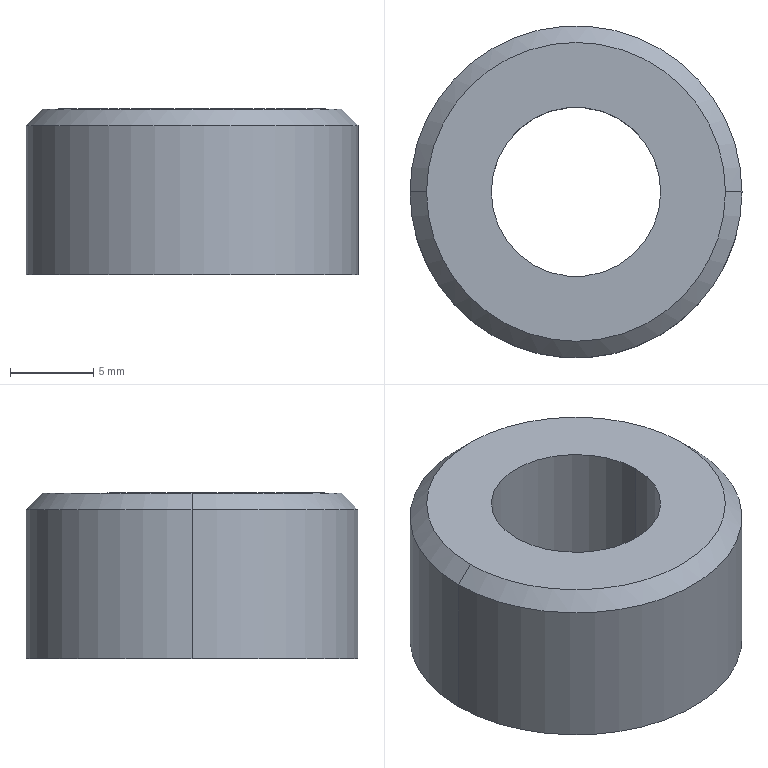Part | SolidWorks | features Chamfer 1, Extrusion 1, HoleWzd 1 | 1 solid | 8 faces | box 20 x 20 x 10 mm | volume 2294 mm3 | cylinder 4 | cone 2 | plane 2 | commonest cylinder face diameters 10.2 x2 20 x2
STEP:
#1=CARTESIAN_POINT('',(9.,0.,10.));
#2=VERTEX_POINT('',#1);
#3=CARTESIAN_POINT('',(-9.,0.,10.));
#4=VERTEX_POINT('',#3);
#5=CARTESIAN_POINT('',(0.,0.,10.));
#6=DIRECTION('',(0.,0.,1.));
#7=DIRECTION('',(1.,0.,0.));
#8=AXIS2_PLACEMENT_3D('',#5,#6,#7);
#9=CIRCLE('',#8,9.);
#10=EDGE_CURVE('',#2,#4,#9,.T.);
#11=ORIENTED_EDGE('',*,*,#10,.F.);
#12=CARTESIAN_POINT('',(10.,0.,9.));
#13=VERTEX_POINT('',#12);
#14=CARTESIAN_POINT('',(9.,0.,10.));
#15=DIRECTION('',(0.7071,0.,-0.7071));
#16=VECTOR('',#15,1000.);
#17=LINE('',#14,#16);
#18=EDGE_CURVE('',#2,#13,#17,.T.);
#19=ORIENTED_EDGE('',*,*,#18,.T.);
#20=CARTESIAN_POINT('',(-10.,0.,9.));
#21=VERTEX_POINT('',#20);
#22=CARTESIAN_POINT('',(0.,0.,9.));
#23=DIRECTION('',(0.,0.,-1.));
#24=DIRECTION('',(1.,0.,0.));
#25=AXIS2_PLACEMENT_3D('',#22,#23,#24);
#26=CIRCLE('',#25,10.);
#27=EDGE_CURVE('',#21,#13,#26,.T.);
#28=ORIENTED_EDGE('',*,*,#27,.F.);
#29=CARTESIAN_POINT('',(-9.,0.,10.));
#30=DIRECTION('',(-0.7071,0.,-0.7071));
#31=VECTOR('',#30,1000.);
#32=LINE('',#29,#31);
#33=EDGE_CURVE('',#4,#21,#32,.T.);
#34=ORIENTED_EDGE('',*,*,#33,.F.);
#35=EDGE_LOOP('',(#11,#19,#28,#34));
#36=FACE_OUTER_BOUND('',#35,.T.);
#37=CARTESIAN_POINT('',(0.,0.,10.));
#38=DIRECTION('',(0.,0.,-1.));
#39=DIRECTION('',(-1.,0.,0.));
#40=AXIS2_PLACEMENT_3D('',#37,#38,#39);
#41=CONICAL_SURFACE('',#40,9.,0.7854);
#42=ADVANCED_FACE('',(#36),#41,.T.);
#43=CARTESIAN_POINT('',(-5.1,0.,0.));
#44=VERTEX_POINT('',#43);
#45=CARTESIAN_POINT('',(5.1,0.,0.));
#46=VERTEX_POINT('',#45);
#47=CARTESIAN_POINT('',(0.,0.,0.));
#48=DIRECTION('',(0.,0.,1.));
#49=DIRECTION('',(1.,0.,0.));
#50=AXIS2_PLACEMENT_3D('',#47,#48,#49);
#51=CIRCLE('',#50,5.1);
#52=EDGE_CURVE('',#44,#46,#51,.T.);
#53=ORIENTED_EDGE('',*,*,#52,.F.);
#54=CARTESIAN_POINT('',(-5.1,0.,10.));
#55=VERTEX_POINT('',#54);
#56=CARTESIAN_POINT('',(-5.1,0.,10.));
#57=DIRECTION('',(0.,0.,1.));
#58=VECTOR('',#57,1000.);
#59=LINE('',#56,#58);
#60=EDGE_CURVE('',#44,#55,#59,.T.);
#61=ORIENTED_EDGE('',*,*,#60,.T.);
#62=CARTESIAN_POINT('',(5.1,0.,10.));
#63=VERTEX_POINT('',#62);
#64=CARTESIAN_POINT('',(0.,0.,10.));
#65=DIRECTION('',(0.,0.,1.));
#66=DIRECTION('',(1.,0.,0.));
#67=AXIS2_PLACEMENT_3D('',#64,#65,#66);
#68=CIRCLE('',#67,5.1);
#69=EDGE_CURVE('',#55,#63,#68,.T.);
#70=ORIENTED_EDGE('',*,*,#69,.T.);
#71=CARTESIAN_POINT('',(5.1,0.,10.));
#72=DIRECTION('',(0.,0.,1.));
#73=VECTOR('',#72,1000.);
#74=LINE('',#71,#73);
#75=EDGE_CURVE('',#46,#63,#74,.T.);
#76=ORIENTED_EDGE('',*,*,#75,.F.);
#77=EDGE_LOOP('',(#53,#61,#70,#76));
#78=FACE_OUTER_BOUND('',#77,.T.);
#79=CARTESIAN_POINT('',(0.,0.,10.));
#80=DIRECTION('',(0.,0.,1.));
#81=DIRECTION('',(1.,0.,0.));
#82=AXIS2_PLACEMENT_3D('',#79,#80,#81);
#83=CYLINDRICAL_SURFACE('',#82,5.1);
#84=ADVANCED_FACE('',(#78),#83,.F.);
#85=ORIENTED_EDGE('',*,*,#27,.T.);
#86=CARTESIAN_POINT('',(10.,0.,0.));
#87=VERTEX_POINT('',#86);
#88=CARTESIAN_POINT('',(10.,0.,10.));
#89=DIRECTION('',(0.,0.,-1.));
#90=VECTOR('',#89,1000.);
#91=LINE('',#88,#90);
#92=EDGE_CURVE('',#13,#87,#91,.T.);
#93=ORIENTED_EDGE('',*,*,#92,.T.);
#94=CARTESIAN_POINT('',(-10.,0.,0.));
#95=VERTEX_POINT('',#94);
#96=CARTESIAN_POINT('',(0.,0.,0.));
#97=DIRECTION('',(0.,0.,1.));
#98=DIRECTION('',(1.,0.,0.));
#99=AXIS2_PLACEMENT_3D('',#96,#97,#98);
#100=CIRCLE('',#99,10.);
#101=EDGE_CURVE('',#87,#95,#100,.T.);
#102=ORIENTED_EDGE('',*,*,#101,.T.);
#103=CARTESIAN_POINT('',(-10.,0.,10.));
#104=DIRECTION('',(0.,0.,-1.));
#105=VECTOR('',#104,1000.);
#106=LINE('',#103,#105);
#107=EDGE_CURVE('',#21,#95,#106,.T.);
#108=ORIENTED_EDGE('',*,*,#107,.F.);
#109=EDGE_LOOP('',(#85,#93,#102,#108));
#110=FACE_OUTER_BOUND('',#109,.T.);
#111=CARTESIAN_POINT('',(0.,0.,10.));
#112=DIRECTION('',(0.,0.,-1.));
#113=DIRECTION('',(-1.,0.,0.));
#114=AXIS2_PLACEMENT_3D('',#111,#112,#113);
#115=CYLINDRICAL_SURFACE('',#114,10.);
#116=ADVANCED_FACE('',(#110),#115,.T.);
#117=ORIENTED_EDGE('',*,*,#92,.F.);
#118=CARTESIAN_POINT('',(0.,0.,9.));
#119=DIRECTION('',(0.,0.,-1.));
#120=DIRECTION('',(1.,0.,0.));
#121=AXIS2_PLACEMENT_3D('',#118,#119,#120);
#122=CIRCLE('',#121,10.);
#123=EDGE_CURVE('',#13,#21,#122,.T.);
#124=ORIENTED_EDGE('',*,*,#123,.T.);
#125=ORIENTED_EDGE('',*,*,#107,.T.);
#126=CARTESIAN_POINT('',(0.,0.,0.));
#127=DIRECTION('',(0.,0.,1.));
#128=DIRECTION('',(1.,0.,0.));
#129=AXIS2_PLACEMENT_3D('',#126,#127,#128);
#130=CIRCLE('',#129,10.);
#131=EDGE_CURVE('',#95,#87,#130,.T.);
#132=ORIENTED_EDGE('',*,*,#131,.T.);
#133=EDGE_LOOP('',(#117,#124,#125,#132));
#134=FACE_OUTER_BOUND('',#133,.T.);
#135=CARTESIAN_POINT('',(0.,0.,10.));
#136=DIRECTION('',(0.,0.,-1.));
#137=DIRECTION('',(-1.,0.,0.));
#138=AXIS2_PLACEMENT_3D('',#135,#136,#137);
#139=CYLINDRICAL_SURFACE('',#138,10.);
#140=ADVANCED_FACE('',(#134),#139,.T.);
#141=CARTESIAN_POINT('',(0.,0.,10.));
#142=DIRECTION('',(0.,0.,1.));
#143=DIRECTION('',(1.,0.,0.));
#144=AXIS2_PLACEMENT_3D('',#141,#142,#143);
#145=CIRCLE('',#144,9.);
#146=EDGE_CURVE('',#4,#2,#145,.T.);
#147=ORIENTED_EDGE('',*,*,#146,.T.);
#148=ORIENTED_EDGE('',*,*,#10,.T.);
#149=EDGE_LOOP('',(#147,#148));
#150=FACE_OUTER_BOUND('',#149,.T.);
#151=CARTESIAN_POINT('',(0.,0.,10.));
#152=DIRECTION('',(0.,0.,1.));
#153=DIRECTION('',(1.,0.,0.));
#154=AXIS2_PLACEMENT_3D('',#151,#152,#153);
#155=CIRCLE('',#154,5.1);
#156=EDGE_CURVE('',#63,#55,#155,.T.);
#157=ORIENTED_EDGE('',*,*,#156,.F.);
#158=ORIENTED_EDGE('',*,*,#69,.F.);
#159=EDGE_LOOP('',(#157,#158));
#160=FACE_BOUND('',#159,.T.);
#161=CARTESIAN_POINT('',(0.,0.,10.));
#162=DIRECTION('',(0.,0.,1.));
#163=DIRECTION('',(1.,0.,0.));
#164=AXIS2_PLACEMENT_3D('',#161,#162,#163);
#165=PLANE('',#164);
#166=ADVANCED_FACE('',(#150,#160),#165,.T.);
#167=CARTESIAN_POINT('',(0.,0.,0.));
#168=DIRECTION('',(0.,0.,1.));
#169=DIRECTION('',(1.,0.,0.));
#170=AXIS2_PLACEMENT_3D('',#167,#168,#169);
#171=CIRCLE('',#170,5.1);
#172=EDGE_CURVE('',#46,#44,#171,.T.);
#173=ORIENTED_EDGE('',*,*,#172,.T.);
#174=ORIENTED_EDGE('',*,*,#52,.T.);
#175=EDGE_LOOP('',(#173,#174));
#176=FACE_BOUND('',#175,.T.);
#177=ORIENTED_EDGE('',*,*,#131,.F.);
#178=ORIENTED_EDGE('',*,*,#101,.F.);
#179=EDGE_LOOP('',(#177,#178));
#180=FACE_OUTER_BOUND('',#179,.T.);
#181=CARTESIAN_POINT('',(0.,0.,0.));
#182=DIRECTION('',(0.,0.,1.));
#183=DIRECTION('',(1.,0.,0.));
#184=AXIS2_PLACEMENT_3D('',#181,#182,#183);
#185=PLANE('',#184);
#186=ADVANCED_FACE('',(#176,#180),#185,.F.);
#187=ORIENTED_EDGE('',*,*,#60,.F.);
#188=ORIENTED_EDGE('',*,*,#172,.F.);
#189=ORIENTED_EDGE('',*,*,#75,.T.);
#190=ORIENTED_EDGE('',*,*,#156,.T.);
#191=EDGE_LOOP('',(#187,#188,#189,#190));
#192=FACE_OUTER_BOUND('',#191,.T.);
#193=CARTESIAN_POINT('',(0.,0.,10.));
#194=DIRECTION('',(0.,0.,1.));
#195=DIRECTION('',(1.,0.,0.));
#196=AXIS2_PLACEMENT_3D('',#193,#194,#195);
#197=CYLINDRICAL_SURFACE('',#196,5.1);
#198=ADVANCED_FACE('',(#192),#197,.F.);
#199=ORIENTED_EDGE('',*,*,#18,.F.);
#200=ORIENTED_EDGE('',*,*,#146,.F.);
#201=ORIENTED_EDGE('',*,*,#33,.T.);
#202=ORIENTED_EDGE('',*,*,#123,.F.);
#203=EDGE_LOOP('',(#199,#200,#201,#202));
#204=FACE_OUTER_BOUND('',#203,.T.);
#205=CARTESIAN_POINT('',(0.,0.,10.));
#206=DIRECTION('',(0.,0.,-1.));
#207=DIRECTION('',(-1.,0.,0.));
#208=AXIS2_PLACEMENT_3D('',#205,#206,#207);
#209=CONICAL_SURFACE('',#208,9.,0.7854);
#210=ADVANCED_FACE('',(#204),#209,.T.);
#211=CLOSED_SHELL('',(#42,#84,#116,#140,#166,#186,#198,#210));
#212=MANIFOLD_SOLID_BREP('',#211);
#213=CARTESIAN_POINT('',(0.,0.,0.));
#214=DIRECTION('',(0.,0.,1.));
#215=DIRECTION('',(1.,0.,0.));
#216=AXIS2_PLACEMENT_3D('',#213,#214,#215);
#217=(LENGTH_UNIT()NAMED_UNIT(*)SI_UNIT(.MILLI.,.METRE.));
#218=UNCERTAINTY_MEASURE_WITH_UNIT(LENGTH_MEASURE(0.00001),#217,'','');
#219=(NAMED_UNIT(*)PLANE_ANGLE_UNIT()SI_UNIT($,.RADIAN.));
#220=(NAMED_UNIT(*)SI_UNIT($,.STERADIAN.)SOLID_ANGLE_UNIT());
#221=(GEOMETRIC_REPRESENTATION_CONTEXT(3)GLOBAL_UNCERTAINTY_ASSIGNED_CONTEXT((#218))GLOBAL_UNIT_ASSIGNED_CONTEXT((#217,#219,#220))REPRESENTATION_CONTEXT('',''));
#222=ADVANCED_BREP_SHAPE_REPRESENTATION('',(#212,#216),#221);